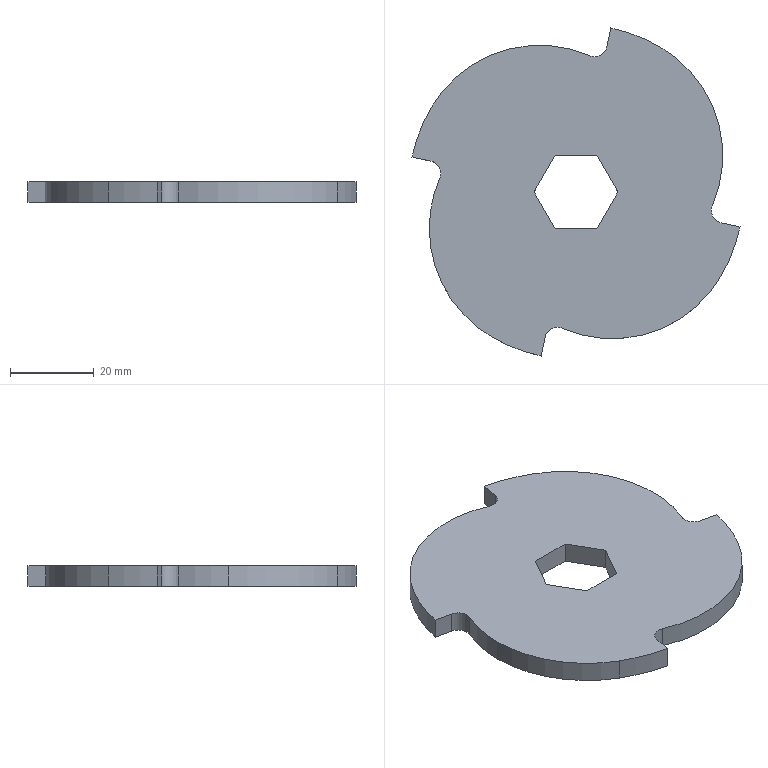Part | NX | 1 solid | 26 faces | box 78.252 x 78.252 x 5 mm | volume 21007 mm3 | cylinder 14 | plane 12 | commonest cylinder face diameters 6 x5 60 x5 80 x4
STEP:
#1=CARTESIAN_POINT('',(-35.,-8.66,5.));
#2=VERTEX_POINT('',#1);
#3=CARTESIAN_POINT('',(-20.,-34.641,5.));
#4=VERTEX_POINT('',#3);
#5=CARTESIAN_POINT('',(-5.,-8.66,5.));
#6=DIRECTION('',(0.,0.,1.));
#7=DIRECTION('',(1.,0.,0.));
#8=AXIS2_PLACEMENT_3D('',#5,#6,#7);
#9=CIRCLE('',#8,30.);
#10=EDGE_CURVE('',#2,#4,#9,.T.);
#11=ORIENTED_EDGE('',*,*,#10,.F.);
#12=CARTESIAN_POINT('',(-35.,-8.66,0.));
#13=VERTEX_POINT('',#12);
#14=CARTESIAN_POINT('',(-35.,-8.66,5.));
#15=DIRECTION('',(0.,0.,-1.));
#16=VECTOR('',#15,1.);
#17=LINE('',#14,#16);
#18=EDGE_CURVE('',#2,#13,#17,.T.);
#19=ORIENTED_EDGE('',*,*,#18,.T.);
#20=CARTESIAN_POINT('',(-20.,-34.641,0.));
#21=VERTEX_POINT('',#20);
#22=CARTESIAN_POINT('',(-5.,-8.66,0.));
#23=DIRECTION('',(0.,0.,1.));
#24=DIRECTION('',(1.,0.,0.));
#25=AXIS2_PLACEMENT_3D('',#22,#23,#24);
#26=CIRCLE('',#25,30.);
#27=EDGE_CURVE('',#13,#21,#26,.T.);
#28=ORIENTED_EDGE('',*,*,#27,.T.);
#29=CARTESIAN_POINT('',(-20.,-34.641,5.));
#30=DIRECTION('',(0.,0.,-1.));
#31=VECTOR('',#30,1.);
#32=LINE('',#29,#31);
#33=EDGE_CURVE('',#4,#21,#32,.T.);
#34=ORIENTED_EDGE('',*,*,#33,.F.);
#35=EDGE_LOOP('',(#11,#19,#28,#34));
#36=FACE_OUTER_BOUND('',#35,.T.);
#37=CARTESIAN_POINT('',(-5.,-8.66,5.));
#38=DIRECTION('',(0.,0.,-1.));
#39=DIRECTION('',(-1.,0.,0.));
#40=AXIS2_PLACEMENT_3D('',#37,#38,#39);
#41=CYLINDRICAL_SURFACE('',#40,30.);
#42=ADVANCED_FACE('',(#36),#41,.T.);
#43=CARTESIAN_POINT('',(32.291,-4.434,5.));
#44=VERTEX_POINT('',#43);
#45=CARTESIAN_POINT('',(32.537,-3.244,5.));
#46=VERTEX_POINT('',#45);
#47=CARTESIAN_POINT('',(35.291,-4.434,5.));
#48=DIRECTION('',(0.,0.,-1.));
#49=DIRECTION('',(1.,0.,0.));
#50=AXIS2_PLACEMENT_3D('',#47,#48,#49);
#51=CIRCLE('',#50,3.);
#52=EDGE_CURVE('',#44,#46,#51,.T.);
#53=ORIENTED_EDGE('',*,*,#52,.F.);
#54=CARTESIAN_POINT('',(32.291,-4.434,0.));
#55=VERTEX_POINT('',#54);
#56=CARTESIAN_POINT('',(32.291,-4.434,5.));
#57=DIRECTION('',(0.,0.,-1.));
#58=VECTOR('',#57,1.);
#59=LINE('',#56,#58);
#60=EDGE_CURVE('',#44,#55,#59,.T.);
#61=ORIENTED_EDGE('',*,*,#60,.T.);
#62=CARTESIAN_POINT('',(32.537,-3.244,0.));
#63=VERTEX_POINT('',#62);
#64=CARTESIAN_POINT('',(35.291,-4.434,0.));
#65=DIRECTION('',(0.,0.,-1.));
#66=DIRECTION('',(1.,0.,0.));
#67=AXIS2_PLACEMENT_3D('',#64,#65,#66);
#68=CIRCLE('',#67,3.);
#69=EDGE_CURVE('',#55,#63,#68,.T.);
#70=ORIENTED_EDGE('',*,*,#69,.T.);
#71=CARTESIAN_POINT('',(32.537,-3.244,5.));
#72=DIRECTION('',(0.,0.,-1.));
#73=VECTOR('',#72,1.);
#74=LINE('',#71,#73);
#75=EDGE_CURVE('',#46,#63,#74,.T.);
#76=ORIENTED_EDGE('',*,*,#75,.F.);
#77=EDGE_LOOP('',(#53,#61,#70,#76));
#78=FACE_OUTER_BOUND('',#77,.T.);
#79=CARTESIAN_POINT('',(35.291,-4.434,5.));
#80=DIRECTION('',(0.,0.,-1.));
#81=DIRECTION('',(-1.,0.,0.));
#82=AXIS2_PLACEMENT_3D('',#79,#80,#81);
#83=CYLINDRICAL_SURFACE('',#82,3.);
#84=ADVANCED_FACE('',(#78),#83,.F.);
#85=CARTESIAN_POINT('',(-3.244,-32.537,0.));
#86=VERTEX_POINT('',#85);
#87=CARTESIAN_POINT('',(34.641,-20.,0.));
#88=VERTEX_POINT('',#87);
#89=CARTESIAN_POINT('',(8.66,-5.,0.));
#90=DIRECTION('',(0.,0.,1.));
#91=DIRECTION('',(1.,0.,0.));
#92=AXIS2_PLACEMENT_3D('',#89,#90,#91);
#93=CIRCLE('',#92,30.);
#94=EDGE_CURVE('',#86,#88,#93,.T.);
#95=ORIENTED_EDGE('',*,*,#94,.T.);
#96=CARTESIAN_POINT('',(34.641,-20.,5.));
#97=VERTEX_POINT('',#96);
#98=CARTESIAN_POINT('',(34.641,-20.,5.));
#99=DIRECTION('',(0.,0.,-1.));
#100=VECTOR('',#99,1.);
#101=LINE('',#98,#100);
#102=EDGE_CURVE('',#97,#88,#101,.T.);
#103=ORIENTED_EDGE('',*,*,#102,.F.);
#104=CARTESIAN_POINT('',(-3.244,-32.537,5.));
#105=VERTEX_POINT('',#104);
#106=CARTESIAN_POINT('',(8.66,-5.,5.));
#107=DIRECTION('',(0.,0.,1.));
#108=DIRECTION('',(1.,0.,0.));
#109=AXIS2_PLACEMENT_3D('',#106,#107,#108);
#110=CIRCLE('',#109,30.);
#111=EDGE_CURVE('',#105,#97,#110,.T.);
#112=ORIENTED_EDGE('',*,*,#111,.F.);
#113=CARTESIAN_POINT('',(-3.244,-32.537,5.));
#114=DIRECTION('',(0.,0.,-1.));
#115=VECTOR('',#114,1.);
#116=LINE('',#113,#115);
#117=EDGE_CURVE('',#105,#86,#116,.T.);
#118=ORIENTED_EDGE('',*,*,#117,.T.);
#119=EDGE_LOOP('',(#95,#103,#112,#118));
#120=FACE_OUTER_BOUND('',#119,.T.);
#121=CARTESIAN_POINT('',(8.66,-5.,5.));
#122=DIRECTION('',(0.,0.,-1.));
#123=DIRECTION('',(-1.,0.,0.));
#124=AXIS2_PLACEMENT_3D('',#121,#122,#123);
#125=CYLINDRICAL_SURFACE('',#124,30.);
#126=ADVANCED_FACE('',(#120),#125,.T.);
#127=CARTESIAN_POINT('',(39.126,-8.316,0.));
#128=VERTEX_POINT('',#127);
#129=CARTESIAN_POINT('',(0.,0.,0.));
#130=DIRECTION('',(0.,0.,1.));
#131=DIRECTION('',(1.,0.,0.));
#132=AXIS2_PLACEMENT_3D('',#129,#130,#131);
#133=CIRCLE('',#132,40.);
#134=EDGE_CURVE('',#88,#128,#133,.T.);
#135=ORIENTED_EDGE('',*,*,#134,.T.);
#136=CARTESIAN_POINT('',(39.126,-8.316,5.));
#137=VERTEX_POINT('',#136);
#138=CARTESIAN_POINT('',(39.126,-8.316,5.));
#139=DIRECTION('',(0.,0.,-1.));
#140=VECTOR('',#139,1.);
#141=LINE('',#138,#140);
#142=EDGE_CURVE('',#137,#128,#141,.T.);
#143=ORIENTED_EDGE('',*,*,#142,.F.);
#144=CARTESIAN_POINT('',(0.,0.,5.));
#145=DIRECTION('',(0.,0.,1.));
#146=DIRECTION('',(1.,0.,0.));
#147=AXIS2_PLACEMENT_3D('',#144,#145,#146);
#148=CIRCLE('',#147,40.);
#149=EDGE_CURVE('',#97,#137,#148,.T.);
#150=ORIENTED_EDGE('',*,*,#149,.F.);
#151=ORIENTED_EDGE('',*,*,#102,.T.);
#152=EDGE_LOOP('',(#135,#143,#150,#151));
#153=FACE_OUTER_BOUND('',#152,.T.);
#154=CARTESIAN_POINT('',(0.,0.,5.));
#155=DIRECTION('',(0.,0.,-1.));
#156=DIRECTION('',(-1.,0.,0.));
#157=AXIS2_PLACEMENT_3D('',#154,#155,#156);
#158=CYLINDRICAL_SURFACE('',#157,40.);
#159=ADVANCED_FACE('',(#153),#158,.T.);
#160=CARTESIAN_POINT('',(34.667,-7.369,0.));
#161=VERTEX_POINT('',#160);
#162=CARTESIAN_POINT('',(17.574,-3.736,0.));
#163=DIRECTION('',(0.9781,-0.2079,0.));
#164=VECTOR('',#163,1.);
#165=LINE('',#162,#164);
#166=EDGE_CURVE('',#161,#128,#165,.T.);
#167=ORIENTED_EDGE('',*,*,#166,.F.);
#168=CARTESIAN_POINT('',(34.667,-7.369,5.));
#169=VERTEX_POINT('',#168);
#170=CARTESIAN_POINT('',(34.667,-7.369,5.));
#171=DIRECTION('',(0.,0.,-1.));
#172=VECTOR('',#171,1.);
#173=LINE('',#170,#172);
#174=EDGE_CURVE('',#169,#161,#173,.T.);
#175=ORIENTED_EDGE('',*,*,#174,.F.);
#176=CARTESIAN_POINT('',(17.574,-3.736,5.));
#177=DIRECTION('',(0.9781,-0.2079,0.));
#178=VECTOR('',#177,1.);
#179=LINE('',#176,#178);
#180=EDGE_CURVE('',#169,#137,#179,.T.);
#181=ORIENTED_EDGE('',*,*,#180,.T.);
#182=ORIENTED_EDGE('',*,*,#142,.T.);
#183=EDGE_LOOP('',(#167,#175,#181,#182));
#184=FACE_OUTER_BOUND('',#183,.T.);
#185=CARTESIAN_POINT('',(17.574,-3.736,5.));
#186=DIRECTION('',(0.2079,0.9781,0.));
#187=DIRECTION('',(-0.9781,0.2079,0.));
#188=AXIS2_PLACEMENT_3D('',#185,#186,#187);
#189=PLANE('',#188);
#190=ADVANCED_FACE('',(#184),#189,.T.);
#191=ORIENTED_EDGE('',*,*,#60,.F.);
#192=CARTESIAN_POINT('',(35.291,-4.434,5.));
#193=DIRECTION('',(0.,0.,-1.));
#194=DIRECTION('',(1.,0.,0.));
#195=AXIS2_PLACEMENT_3D('',#192,#193,#194);
#196=CIRCLE('',#195,3.);
#197=EDGE_CURVE('',#169,#44,#196,.T.);
#198=ORIENTED_EDGE('',*,*,#197,.F.);
#199=ORIENTED_EDGE('',*,*,#174,.T.);
#200=CARTESIAN_POINT('',(35.291,-4.434,0.));
#201=DIRECTION('',(0.,0.,-1.));
#202=DIRECTION('',(1.,0.,0.));
#203=AXIS2_PLACEMENT_3D('',#200,#201,#202);
#204=CIRCLE('',#203,3.);
#205=EDGE_CURVE('',#161,#55,#204,.T.);
#206=ORIENTED_EDGE('',*,*,#205,.T.);
#207=EDGE_LOOP('',(#191,#198,#199,#206));
#208=FACE_OUTER_BOUND('',#207,.T.);
#209=CARTESIAN_POINT('',(35.291,-4.434,5.));
#210=DIRECTION('',(0.,0.,-1.));
#211=DIRECTION('',(-1.,0.,0.));
#212=AXIS2_PLACEMENT_3D('',#209,#210,#211);
#213=CYLINDRICAL_SURFACE('',#212,3.);
#214=ADVANCED_FACE('',(#208),#213,.F.);
#215=CARTESIAN_POINT('',(20.,34.641,0.));
#216=VERTEX_POINT('',#215);
#217=CARTESIAN_POINT('',(5.,8.66,0.));
#218=DIRECTION('',(0.,0.,1.));
#219=DIRECTION('',(1.,0.,0.));
#220=AXIS2_PLACEMENT_3D('',#217,#218,#219);
#221=CIRCLE('',#220,30.);
#222=EDGE_CURVE('',#63,#216,#221,.T.);
#223=ORIENTED_EDGE('',*,*,#222,.T.);
#224=CARTESIAN_POINT('',(20.,34.641,5.));
#225=VERTEX_POINT('',#224);
#226=CARTESIAN_POINT('',(20.,34.641,5.));
#227=DIRECTION('',(0.,0.,-1.));
#228=VECTOR('',#227,1.);
#229=LINE('',#226,#228);
#230=EDGE_CURVE('',#225,#216,#229,.T.);
#231=ORIENTED_EDGE('',*,*,#230,.F.);
#232=CARTESIAN_POINT('',(5.,8.66,5.));
#233=DIRECTION('',(0.,0.,1.));
#234=DIRECTION('',(1.,0.,0.));
#235=AXIS2_PLACEMENT_3D('',#232,#233,#234);
#236=CIRCLE('',#235,30.);
#237=EDGE_CURVE('',#46,#225,#236,.T.);
#238=ORIENTED_EDGE('',*,*,#237,.F.);
#239=ORIENTED_EDGE('',*,*,#75,.T.);
#240=EDGE_LOOP('',(#223,#231,#238,#239));
#241=FACE_OUTER_BOUND('',#240,.T.);
#242=CARTESIAN_POINT('',(5.,8.66,5.));
#243=DIRECTION('',(0.,0.,-1.));
#244=DIRECTION('',(-1.,0.,0.));
#245=AXIS2_PLACEMENT_3D('',#242,#243,#244);
#246=CYLINDRICAL_SURFACE('',#245,30.);
#247=ADVANCED_FACE('',(#241),#246,.T.);
#248=CARTESIAN_POINT('',(8.316,39.126,0.));
#249=VERTEX_POINT('',#248);
#250=CARTESIAN_POINT('',(0.,0.,0.));
#251=DIRECTION('',(0.,0.,1.));
#252=DIRECTION('',(1.,0.,0.));
#253=AXIS2_PLACEMENT_3D('',#250,#251,#252);
#254=CIRCLE('',#253,40.);
#255=EDGE_CURVE('',#216,#249,#254,.T.);
#256=ORIENTED_EDGE('',*,*,#255,.T.);
#257=CARTESIAN_POINT('',(8.316,39.126,5.));
#258=VERTEX_POINT('',#257);
#259=CARTESIAN_POINT('',(8.316,39.126,5.));
#260=DIRECTION('',(0.,0.,-1.));
#261=VECTOR('',#260,1.);
#262=LINE('',#259,#261);
#263=EDGE_CURVE('',#258,#249,#262,.T.);
#264=ORIENTED_EDGE('',*,*,#263,.F.);
#265=CARTESIAN_POINT('',(0.,0.,5.));
#266=DIRECTION('',(0.,0.,1.));
#267=DIRECTION('',(1.,0.,0.));
#268=AXIS2_PLACEMENT_3D('',#265,#266,#267);
#269=CIRCLE('',#268,40.);
#270=EDGE_CURVE('',#225,#258,#269,.T.);
#271=ORIENTED_EDGE('',*,*,#270,.F.);
#272=ORIENTED_EDGE('',*,*,#230,.T.);
#273=EDGE_LOOP('',(#256,#264,#271,#272));
#274=FACE_OUTER_BOUND('',#273,.T.);
#275=CARTESIAN_POINT('',(0.,0.,5.));
#276=DIRECTION('',(0.,0.,-1.));
#277=DIRECTION('',(-1.,0.,0.));
#278=AXIS2_PLACEMENT_3D('',#275,#276,#277);
#279=CYLINDRICAL_SURFACE('',#278,40.);
#280=ADVANCED_FACE('',(#274),#279,.T.);
#281=CARTESIAN_POINT('',(7.369,34.667,0.));
#282=VERTEX_POINT('',#281);
#283=CARTESIAN_POINT('',(-17.016,-80.056,0.));
#284=DIRECTION('',(0.2079,0.9781,0.));
#285=VECTOR('',#284,1.);
#286=LINE('',#283,#285);
#287=EDGE_CURVE('',#282,#249,#286,.T.);
#288=ORIENTED_EDGE('',*,*,#287,.F.);
#289=CARTESIAN_POINT('',(7.369,34.667,5.));
#290=VERTEX_POINT('',#289);
#291=CARTESIAN_POINT('',(7.369,34.667,5.));
#292=DIRECTION('',(0.,0.,-1.));
#293=VECTOR('',#292,1.);
#294=LINE('',#291,#293);
#295=EDGE_CURVE('',#290,#282,#294,.T.);
#296=ORIENTED_EDGE('',*,*,#295,.F.);
#297=CARTESIAN_POINT('',(-17.016,-80.056,5.));
#298=DIRECTION('',(0.2079,0.9781,0.));
#299=VECTOR('',#298,1.);
#300=LINE('',#297,#299);
#301=EDGE_CURVE('',#290,#258,#300,.T.);
#302=ORIENTED_EDGE('',*,*,#301,.T.);
#303=ORIENTED_EDGE('',*,*,#263,.T.);
#304=EDGE_LOOP('',(#288,#296,#302,#303));
#305=FACE_OUTER_BOUND('',#304,.T.);
#306=CARTESIAN_POINT('',(-17.016,-80.056,5.));
#307=DIRECTION('',(-0.9781,0.2079,0.));
#308=DIRECTION('',(-0.2079,-0.9781,0.));
#309=AXIS2_PLACEMENT_3D('',#306,#307,#308);
#310=PLANE('',#309);
#311=ADVANCED_FACE('',(#305),#310,.T.);
#312=CARTESIAN_POINT('',(3.244,32.537,0.));
#313=VERTEX_POINT('',#312);
#314=CARTESIAN_POINT('',(4.434,35.291,0.));
#315=DIRECTION('',(0.,0.,-1.));
#316=DIRECTION('',(1.,0.,0.));
#317=AXIS2_PLACEMENT_3D('',#314,#315,#316);
#318=CIRCLE('',#317,3.);
#319=EDGE_CURVE('',#282,#313,#318,.T.);
#320=ORIENTED_EDGE('',*,*,#319,.T.);
#321=CARTESIAN_POINT('',(3.244,32.537,5.));
#322=VERTEX_POINT('',#321);
#323=CARTESIAN_POINT('',(3.244,32.537,5.));
#324=DIRECTION('',(0.,0.,-1.));
#325=VECTOR('',#324,1.);
#326=LINE('',#323,#325);
#327=EDGE_CURVE('',#322,#313,#326,.T.);
#328=ORIENTED_EDGE('',*,*,#327,.F.);
#329=CARTESIAN_POINT('',(4.434,35.291,5.));
#330=DIRECTION('',(0.,0.,-1.));
#331=DIRECTION('',(1.,0.,0.));
#332=AXIS2_PLACEMENT_3D('',#329,#330,#331);
#333=CIRCLE('',#332,3.);
#334=EDGE_CURVE('',#290,#322,#333,.T.);
#335=ORIENTED_EDGE('',*,*,#334,.F.);
#336=ORIENTED_EDGE('',*,*,#295,.T.);
#337=EDGE_LOOP('',(#320,#328,#335,#336));
#338=FACE_OUTER_BOUND('',#337,.T.);
#339=CARTESIAN_POINT('',(4.434,35.291,5.));
#340=DIRECTION('',(0.,0.,-1.));
#341=DIRECTION('',(-1.,0.,0.));
#342=AXIS2_PLACEMENT_3D('',#339,#340,#341);
#343=CYLINDRICAL_SURFACE('',#342,3.);
#344=ADVANCED_FACE('',(#338),#343,.F.);
#345=CARTESIAN_POINT('',(-34.641,20.,0.));
#346=VERTEX_POINT('',#345);
#347=CARTESIAN_POINT('',(-8.66,5.,0.));
#348=DIRECTION('',(0.,0.,1.));
#349=DIRECTION('',(1.,0.,0.));
#350=AXIS2_PLACEMENT_3D('',#347,#348,#349);
#351=CIRCLE('',#350,30.);
#352=EDGE_CURVE('',#313,#346,#351,.T.);
#353=ORIENTED_EDGE('',*,*,#352,.T.);
#354=CARTESIAN_POINT('',(-34.641,20.,5.));
#355=VERTEX_POINT('',#354);
#356=CARTESIAN_POINT('',(-34.641,20.,5.));
#357=DIRECTION('',(0.,0.,-1.));
#358=VECTOR('',#357,1.);
#359=LINE('',#356,#358);
#360=EDGE_CURVE('',#355,#346,#359,.T.);
#361=ORIENTED_EDGE('',*,*,#360,.F.);
#362=CARTESIAN_POINT('',(-8.66,5.,5.));
#363=DIRECTION('',(0.,0.,1.));
#364=DIRECTION('',(1.,0.,0.));
#365=AXIS2_PLACEMENT_3D('',#362,#363,#364);
#366=CIRCLE('',#365,30.);
#367=EDGE_CURVE('',#322,#355,#366,.T.);
#368=ORIENTED_EDGE('',*,*,#367,.F.);
#369=ORIENTED_EDGE('',*,*,#327,.T.);
#370=EDGE_LOOP('',(#353,#361,#368,#369));
#371=FACE_OUTER_BOUND('',#370,.T.);
#372=CARTESIAN_POINT('',(-8.66,5.,5.));
#373=DIRECTION('',(0.,0.,-1.));
#374=DIRECTION('',(-1.,0.,0.));
#375=AXIS2_PLACEMENT_3D('',#372,#373,#374);
#376=CYLINDRICAL_SURFACE('',#375,30.);
#377=ADVANCED_FACE('',(#371),#376,.T.);
#378=CARTESIAN_POINT('',(-39.126,8.316,0.));
#379=VERTEX_POINT('',#378);
#380=CARTESIAN_POINT('',(0.,0.,0.));
#381=DIRECTION('',(0.,0.,1.));
#382=DIRECTION('',(1.,0.,0.));
#383=AXIS2_PLACEMENT_3D('',#380,#381,#382);
#384=CIRCLE('',#383,40.);
#385=EDGE_CURVE('',#346,#379,#384,.T.);
#386=ORIENTED_EDGE('',*,*,#385,.T.);
#387=CARTESIAN_POINT('',(-39.126,8.316,5.));
#388=VERTEX_POINT('',#387);
#389=CARTESIAN_POINT('',(-39.126,8.316,5.));
#390=DIRECTION('',(0.,0.,-1.));
#391=VECTOR('',#390,1.);
#392=LINE('',#389,#391);
#393=EDGE_CURVE('',#388,#379,#392,.T.);
#394=ORIENTED_EDGE('',*,*,#393,.F.);
#395=CARTESIAN_POINT('',(0.,0.,5.));
#396=DIRECTION('',(0.,0.,1.));
#397=DIRECTION('',(1.,0.,0.));
#398=AXIS2_PLACEMENT_3D('',#395,#396,#397);
#399=CIRCLE('',#398,40.);
#400=EDGE_CURVE('',#355,#388,#399,.T.);
#401=ORIENTED_EDGE('',*,*,#400,.F.);
#402=ORIENTED_EDGE('',*,*,#360,.T.);
#403=EDGE_LOOP('',(#386,#394,#401,#402));
#404=FACE_OUTER_BOUND('',#403,.T.);
#405=CARTESIAN_POINT('',(0.,0.,5.));
#406=DIRECTION('',(0.,0.,-1.));
#407=DIRECTION('',(-1.,0.,0.));
#408=AXIS2_PLACEMENT_3D('',#405,#406,#407);
#409=CYLINDRICAL_SURFACE('',#408,40.);
#410=ADVANCED_FACE('',(#404),#409,.T.);
#411=CARTESIAN_POINT('',(-34.667,7.369,0.));
#412=VERTEX_POINT('',#411);
#413=CARTESIAN_POINT('',(17.574,-3.736,0.));
#414=DIRECTION('',(-0.9781,0.2079,0.));
#415=VECTOR('',#414,1.);
#416=LINE('',#413,#415);
#417=EDGE_CURVE('',#412,#379,#416,.T.);
#418=ORIENTED_EDGE('',*,*,#417,.F.);
#419=CARTESIAN_POINT('',(-34.667,7.369,5.));
#420=VERTEX_POINT('',#419);
#421=CARTESIAN_POINT('',(-34.667,7.369,5.));
#422=DIRECTION('',(0.,0.,-1.));
#423=VECTOR('',#422,1.);
#424=LINE('',#421,#423);
#425=EDGE_CURVE('',#420,#412,#424,.T.);
#426=ORIENTED_EDGE('',*,*,#425,.F.);
#427=CARTESIAN_POINT('',(17.574,-3.736,5.));
#428=DIRECTION('',(-0.9781,0.2079,0.));
#429=VECTOR('',#428,1.);
#430=LINE('',#427,#429);
#431=EDGE_CURVE('',#420,#388,#430,.T.);
#432=ORIENTED_EDGE('',*,*,#431,.T.);
#433=ORIENTED_EDGE('',*,*,#393,.T.);
#434=EDGE_LOOP('',(#418,#426,#432,#433));
#435=FACE_OUTER_BOUND('',#434,.T.);
#436=CARTESIAN_POINT('',(17.574,-3.736,5.));
#437=DIRECTION('',(-0.2079,-0.9781,0.));
#438=DIRECTION('',(0.9781,-0.2079,0.));
#439=AXIS2_PLACEMENT_3D('',#436,#437,#438);
#440=PLANE('',#439);
#441=ADVANCED_FACE('',(#435),#440,.T.);
#442=CARTESIAN_POINT('',(-32.537,3.244,0.));
#443=VERTEX_POINT('',#442);
#444=CARTESIAN_POINT('',(-35.291,4.434,0.));
#445=DIRECTION('',(0.,0.,-1.));
#446=DIRECTION('',(1.,0.,0.));
#447=AXIS2_PLACEMENT_3D('',#444,#445,#446);
#448=CIRCLE('',#447,3.);
#449=EDGE_CURVE('',#412,#443,#448,.T.);
#450=ORIENTED_EDGE('',*,*,#449,.T.);
#451=CARTESIAN_POINT('',(-32.537,3.244,5.));
#452=VERTEX_POINT('',#451);
#453=CARTESIAN_POINT('',(-32.537,3.244,5.));
#454=DIRECTION('',(0.,0.,-1.));
#455=VECTOR('',#454,1.);
#456=LINE('',#453,#455);
#457=EDGE_CURVE('',#452,#443,#456,.T.);
#458=ORIENTED_EDGE('',*,*,#457,.F.);
#459=CARTESIAN_POINT('',(-35.291,4.434,5.));
#460=DIRECTION('',(0.,0.,-1.));
#461=DIRECTION('',(1.,0.,0.));
#462=AXIS2_PLACEMENT_3D('',#459,#460,#461);
#463=CIRCLE('',#462,3.);
#464=EDGE_CURVE('',#420,#452,#463,.T.);
#465=ORIENTED_EDGE('',*,*,#464,.F.);
#466=ORIENTED_EDGE('',*,*,#425,.T.);
#467=EDGE_LOOP('',(#450,#458,#465,#466));
#468=FACE_OUTER_BOUND('',#467,.T.);
#469=CARTESIAN_POINT('',(-35.291,4.434,5.));
#470=DIRECTION('',(0.,0.,-1.));
#471=DIRECTION('',(-1.,0.,0.));
#472=AXIS2_PLACEMENT_3D('',#469,#470,#471);
#473=CYLINDRICAL_SURFACE('',#472,3.);
#474=ADVANCED_FACE('',(#468),#473,.F.);
#475=ORIENTED_EDGE('',*,*,#18,.F.);
#476=CARTESIAN_POINT('',(-5.,-8.66,5.));
#477=DIRECTION('',(0.,0.,1.));
#478=DIRECTION('',(1.,0.,0.));
#479=AXIS2_PLACEMENT_3D('',#476,#477,#478);
#480=CIRCLE('',#479,30.);
#481=EDGE_CURVE('',#452,#2,#480,.T.);
#482=ORIENTED_EDGE('',*,*,#481,.F.);
#483=ORIENTED_EDGE('',*,*,#457,.T.);
#484=CARTESIAN_POINT('',(-5.,-8.66,0.));
#485=DIRECTION('',(0.,0.,1.));
#486=DIRECTION('',(1.,0.,0.));
#487=AXIS2_PLACEMENT_3D('',#484,#485,#486);
#488=CIRCLE('',#487,30.);
#489=EDGE_CURVE('',#443,#13,#488,.T.);
#490=ORIENTED_EDGE('',*,*,#489,.T.);
#491=EDGE_LOOP('',(#475,#482,#483,#490));
#492=FACE_OUTER_BOUND('',#491,.T.);
#493=CARTESIAN_POINT('',(-5.,-8.66,5.));
#494=DIRECTION('',(0.,0.,-1.));
#495=DIRECTION('',(-1.,0.,0.));
#496=AXIS2_PLACEMENT_3D('',#493,#494,#495);
#497=CYLINDRICAL_SURFACE('',#496,30.);
#498=ADVANCED_FACE('',(#492),#497,.T.);
#499=CARTESIAN_POINT('',(-8.316,-39.126,0.));
#500=VERTEX_POINT('',#499);
#501=CARTESIAN_POINT('',(0.,0.,0.));
#502=DIRECTION('',(0.,0.,1.));
#503=DIRECTION('',(1.,0.,0.));
#504=AXIS2_PLACEMENT_3D('',#501,#502,#503);
#505=CIRCLE('',#504,40.);
#506=EDGE_CURVE('',#21,#500,#505,.T.);
#507=ORIENTED_EDGE('',*,*,#506,.T.);
#508=CARTESIAN_POINT('',(-8.316,-39.126,5.));
#509=VERTEX_POINT('',#508);
#510=CARTESIAN_POINT('',(-8.316,-39.126,5.));
#511=DIRECTION('',(0.,0.,-1.));
#512=VECTOR('',#511,1.);
#513=LINE('',#510,#512);
#514=EDGE_CURVE('',#509,#500,#513,.T.);
#515=ORIENTED_EDGE('',*,*,#514,.F.);
#516=CARTESIAN_POINT('',(0.,0.,5.));
#517=DIRECTION('',(0.,0.,1.));
#518=DIRECTION('',(1.,0.,0.));
#519=AXIS2_PLACEMENT_3D('',#516,#517,#518);
#520=CIRCLE('',#519,40.);
#521=EDGE_CURVE('',#4,#509,#520,.T.);
#522=ORIENTED_EDGE('',*,*,#521,.F.);
#523=ORIENTED_EDGE('',*,*,#33,.T.);
#524=EDGE_LOOP('',(#507,#515,#522,#523));
#525=FACE_OUTER_BOUND('',#524,.T.);
#526=CARTESIAN_POINT('',(0.,0.,5.));
#527=DIRECTION('',(0.,0.,-1.));
#528=DIRECTION('',(-1.,0.,0.));
#529=AXIS2_PLACEMENT_3D('',#526,#527,#528);
#530=CYLINDRICAL_SURFACE('',#529,40.);
#531=ADVANCED_FACE('',(#525),#530,.T.);
#532=CARTESIAN_POINT('',(-7.369,-34.667,0.));
#533=VERTEX_POINT('',#532);
#534=CARTESIAN_POINT('',(-17.016,-80.056,0.));
#535=DIRECTION('',(-0.2079,-0.9781,0.));
#536=VECTOR('',#535,1.);
#537=LINE('',#534,#536);
#538=EDGE_CURVE('',#533,#500,#537,.T.);
#539=ORIENTED_EDGE('',*,*,#538,.F.);
#540=CARTESIAN_POINT('',(-7.369,-34.667,5.));
#541=VERTEX_POINT('',#540);
#542=CARTESIAN_POINT('',(-7.369,-34.667,5.));
#543=DIRECTION('',(0.,0.,-1.));
#544=VECTOR('',#543,1.);
#545=LINE('',#542,#544);
#546=EDGE_CURVE('',#541,#533,#545,.T.);
#547=ORIENTED_EDGE('',*,*,#546,.F.);
#548=CARTESIAN_POINT('',(-17.016,-80.056,5.));
#549=DIRECTION('',(-0.2079,-0.9781,0.));
#550=VECTOR('',#549,1.);
#551=LINE('',#548,#550);
#552=EDGE_CURVE('',#541,#509,#551,.T.);
#553=ORIENTED_EDGE('',*,*,#552,.T.);
#554=ORIENTED_EDGE('',*,*,#514,.T.);
#555=EDGE_LOOP('',(#539,#547,#553,#554));
#556=FACE_OUTER_BOUND('',#555,.T.);
#557=CARTESIAN_POINT('',(-17.016,-80.056,5.));
#558=DIRECTION('',(0.9781,-0.2079,0.));
#559=DIRECTION('',(0.2079,0.9781,0.));
#560=AXIS2_PLACEMENT_3D('',#557,#558,#559);
#561=PLANE('',#560);
#562=ADVANCED_FACE('',(#556),#561,.T.);
#563=CARTESIAN_POINT('',(5.,-8.66,0.));
#564=VERTEX_POINT('',#563);
#565=CARTESIAN_POINT('',(10.,0.,0.));
#566=VERTEX_POINT('',#565);
#567=CARTESIAN_POINT('',(-28.643,-66.932,0.));
#568=DIRECTION('',(0.5,0.866,0.));
#569=VECTOR('',#568,1.);
#570=LINE('',#567,#569);
#571=EDGE_CURVE('',#564,#566,#570,.T.);
#572=ORIENTED_EDGE('',*,*,#571,.F.);
#573=CARTESIAN_POINT('',(5.,-8.66,5.));
#574=VERTEX_POINT('',#573);
#575=CARTESIAN_POINT('',(5.,-8.66,5.));
#576=DIRECTION('',(0.,0.,-1.));
#577=VECTOR('',#576,1.);
#578=LINE('',#575,#577);
#579=EDGE_CURVE('',#574,#564,#578,.T.);
#580=ORIENTED_EDGE('',*,*,#579,.F.);
#581=CARTESIAN_POINT('',(10.,0.,5.));
#582=VERTEX_POINT('',#581);
#583=CARTESIAN_POINT('',(-28.643,-66.932,5.));
#584=DIRECTION('',(0.5,0.866,0.));
#585=VECTOR('',#584,1.);
#586=LINE('',#583,#585);
#587=EDGE_CURVE('',#574,#582,#586,.T.);
#588=ORIENTED_EDGE('',*,*,#587,.T.);
#589=CARTESIAN_POINT('',(10.,0.,5.));
#590=DIRECTION('',(0.,0.,-1.));
#591=VECTOR('',#590,1.);
#592=LINE('',#589,#591);
#593=EDGE_CURVE('',#582,#566,#592,.T.);
#594=ORIENTED_EDGE('',*,*,#593,.T.);
#595=EDGE_LOOP('',(#572,#580,#588,#594));
#596=FACE_OUTER_BOUND('',#595,.T.);
#597=CARTESIAN_POINT('',(-28.643,-66.932,5.));
#598=DIRECTION('',(-0.866,0.5,0.));
#599=DIRECTION('',(-0.5,-0.866,0.));
#600=AXIS2_PLACEMENT_3D('',#597,#598,#599);
#601=PLANE('',#600);
#602=ADVANCED_FACE('',(#596),#601,.T.);
#603=CARTESIAN_POINT('',(-5.,-8.66,0.));
#604=VERTEX_POINT('',#603);
#605=CARTESIAN_POINT('',(0.5581,-8.66,0.));
#606=DIRECTION('',(1.,0.,0.));
#607=VECTOR('',#606,1.);
#608=LINE('',#605,#607);
#609=EDGE_CURVE('',#604,#564,#608,.T.);
#610=ORIENTED_EDGE('',*,*,#609,.F.);
#611=CARTESIAN_POINT('',(-5.,-8.66,5.));
#612=VERTEX_POINT('',#611);
#613=CARTESIAN_POINT('',(-5.,-8.66,5.));
#614=DIRECTION('',(0.,0.,-1.));
#615=VECTOR('',#614,1.);
#616=LINE('',#613,#615);
#617=EDGE_CURVE('',#612,#604,#616,.T.);
#618=ORIENTED_EDGE('',*,*,#617,.F.);
#619=CARTESIAN_POINT('',(0.5581,-8.66,5.));
#620=DIRECTION('',(1.,0.,0.));
#621=VECTOR('',#620,1.);
#622=LINE('',#619,#621);
#623=EDGE_CURVE('',#612,#574,#622,.T.);
#624=ORIENTED_EDGE('',*,*,#623,.T.);
#625=ORIENTED_EDGE('',*,*,#579,.T.);
#626=EDGE_LOOP('',(#610,#618,#624,#625));
#627=FACE_OUTER_BOUND('',#626,.T.);
#628=CARTESIAN_POINT('',(0.5581,-8.66,5.));
#629=DIRECTION('',(0.,1.,0.));
#630=DIRECTION('',(-1.,0.,0.));
#631=AXIS2_PLACEMENT_3D('',#628,#629,#630);
#632=PLANE('',#631);
#633=ADVANCED_FACE('',(#627),#632,.T.);
#634=CARTESIAN_POINT('',(-10.,0.,0.));
#635=VERTEX_POINT('',#634);
#636=CARTESIAN_POINT('',(28.922,-67.415,0.));
#637=DIRECTION('',(0.5,-0.866,0.));
#638=VECTOR('',#637,1.);
#639=LINE('',#636,#638);
#640=EDGE_CURVE('',#635,#604,#639,.T.);
#641=ORIENTED_EDGE('',*,*,#640,.F.);
#642=CARTESIAN_POINT('',(-10.,0.,5.));
#643=VERTEX_POINT('',#642);
#644=CARTESIAN_POINT('',(-10.,0.,5.));
#645=DIRECTION('',(0.,0.,-1.));
#646=VECTOR('',#645,1.);
#647=LINE('',#644,#646);
#648=EDGE_CURVE('',#643,#635,#647,.T.);
#649=ORIENTED_EDGE('',*,*,#648,.F.);
#650=CARTESIAN_POINT('',(28.922,-67.415,5.));
#651=DIRECTION('',(0.5,-0.866,0.));
#652=VECTOR('',#651,1.);
#653=LINE('',#650,#652);
#654=EDGE_CURVE('',#643,#612,#653,.T.);
#655=ORIENTED_EDGE('',*,*,#654,.T.);
#656=ORIENTED_EDGE('',*,*,#617,.T.);
#657=EDGE_LOOP('',(#641,#649,#655,#656));
#658=FACE_OUTER_BOUND('',#657,.T.);
#659=CARTESIAN_POINT('',(28.922,-67.415,5.));
#660=DIRECTION('',(0.866,0.5,0.));
#661=DIRECTION('',(-0.5,0.866,0.));
#662=AXIS2_PLACEMENT_3D('',#659,#660,#661);
#663=PLANE('',#662);
#664=ADVANCED_FACE('',(#658),#663,.T.);
#665=CARTESIAN_POINT('',(-5.,8.66,0.));
#666=VERTEX_POINT('',#665);
#667=CARTESIAN_POINT('',(-43.643,-58.272,0.));
#668=DIRECTION('',(-0.5,-0.866,0.));
#669=VECTOR('',#668,1.);
#670=LINE('',#667,#669);
#671=EDGE_CURVE('',#666,#635,#670,.T.);
#672=ORIENTED_EDGE('',*,*,#671,.F.);
#673=CARTESIAN_POINT('',(-5.,8.66,5.));
#674=VERTEX_POINT('',#673);
#675=CARTESIAN_POINT('',(-5.,8.66,5.));
#676=DIRECTION('',(0.,0.,-1.));
#677=VECTOR('',#676,1.);
#678=LINE('',#675,#677);
#679=EDGE_CURVE('',#674,#666,#678,.T.);
#680=ORIENTED_EDGE('',*,*,#679,.F.);
#681=CARTESIAN_POINT('',(-43.643,-58.272,5.));
#682=DIRECTION('',(-0.5,-0.866,0.));
#683=VECTOR('',#682,1.);
#684=LINE('',#681,#683);
#685=EDGE_CURVE('',#674,#643,#684,.T.);
#686=ORIENTED_EDGE('',*,*,#685,.T.);
#687=ORIENTED_EDGE('',*,*,#648,.T.);
#688=EDGE_LOOP('',(#672,#680,#686,#687));
#689=FACE_OUTER_BOUND('',#688,.T.);
#690=CARTESIAN_POINT('',(-43.643,-58.272,5.));
#691=DIRECTION('',(0.866,-0.5,0.));
#692=DIRECTION('',(0.5,0.866,0.));
#693=AXIS2_PLACEMENT_3D('',#690,#691,#692);
#694=PLANE('',#693);
#695=ADVANCED_FACE('',(#689),#694,.T.);
#696=CARTESIAN_POINT('',(5.,8.66,0.));
#697=VERTEX_POINT('',#696);
#698=CARTESIAN_POINT('',(0.5581,8.66,0.));
#699=DIRECTION('',(-1.,0.,0.));
#700=VECTOR('',#699,1.);
#701=LINE('',#698,#700);
#702=EDGE_CURVE('',#697,#666,#701,.T.);
#703=ORIENTED_EDGE('',*,*,#702,.F.);
#704=CARTESIAN_POINT('',(5.,8.66,5.));
#705=VERTEX_POINT('',#704);
#706=CARTESIAN_POINT('',(5.,8.66,5.));
#707=DIRECTION('',(0.,0.,-1.));
#708=VECTOR('',#707,1.);
#709=LINE('',#706,#708);
#710=EDGE_CURVE('',#705,#697,#709,.T.);
#711=ORIENTED_EDGE('',*,*,#710,.F.);
#712=CARTESIAN_POINT('',(0.5581,8.66,5.));
#713=DIRECTION('',(-1.,0.,0.));
#714=VECTOR('',#713,1.);
#715=LINE('',#712,#714);
#716=EDGE_CURVE('',#705,#674,#715,.T.);
#717=ORIENTED_EDGE('',*,*,#716,.T.);
#718=ORIENTED_EDGE('',*,*,#679,.T.);
#719=EDGE_LOOP('',(#703,#711,#717,#718));
#720=FACE_OUTER_BOUND('',#719,.T.);
#721=CARTESIAN_POINT('',(0.5581,8.66,5.));
#722=DIRECTION('',(0.,-1.,0.));
#723=DIRECTION('',(1.,0.,0.));
#724=AXIS2_PLACEMENT_3D('',#721,#722,#723);
#725=PLANE('',#724);
#726=ADVANCED_FACE('',(#720),#725,.T.);
#727=CARTESIAN_POINT('',(43.922,-58.755,0.));
#728=DIRECTION('',(-0.5,0.866,0.));
#729=VECTOR('',#728,1.);
#730=LINE('',#727,#729);
#731=EDGE_CURVE('',#566,#697,#730,.T.);
#732=ORIENTED_EDGE('',*,*,#731,.F.);
#733=ORIENTED_EDGE('',*,*,#593,.F.);
#734=CARTESIAN_POINT('',(43.922,-58.755,5.));
#735=DIRECTION('',(-0.5,0.866,0.));
#736=VECTOR('',#735,1.);
#737=LINE('',#734,#736);
#738=EDGE_CURVE('',#582,#705,#737,.T.);
#739=ORIENTED_EDGE('',*,*,#738,.T.);
#740=ORIENTED_EDGE('',*,*,#710,.T.);
#741=EDGE_LOOP('',(#732,#733,#739,#740));
#742=FACE_OUTER_BOUND('',#741,.T.);
#743=CARTESIAN_POINT('',(43.922,-58.755,5.));
#744=DIRECTION('',(-0.866,-0.5,0.));
#745=DIRECTION('',(0.5,-0.866,0.));
#746=AXIS2_PLACEMENT_3D('',#743,#744,#745);
#747=PLANE('',#746);
#748=ADVANCED_FACE('',(#742),#747,.T.);
#749=CARTESIAN_POINT('',(-4.434,-35.291,0.));
#750=DIRECTION('',(0.,0.,-1.));
#751=DIRECTION('',(1.,0.,0.));
#752=AXIS2_PLACEMENT_3D('',#749,#750,#751);
#753=CIRCLE('',#752,3.);
#754=EDGE_CURVE('',#533,#86,#753,.T.);
#755=ORIENTED_EDGE('',*,*,#754,.T.);
#756=ORIENTED_EDGE('',*,*,#117,.F.);
#757=CARTESIAN_POINT('',(-4.434,-35.291,5.));
#758=DIRECTION('',(0.,0.,-1.));
#759=DIRECTION('',(1.,0.,0.));
#760=AXIS2_PLACEMENT_3D('',#757,#758,#759);
#761=CIRCLE('',#760,3.);
#762=EDGE_CURVE('',#541,#105,#761,.T.);
#763=ORIENTED_EDGE('',*,*,#762,.F.);
#764=ORIENTED_EDGE('',*,*,#546,.T.);
#765=EDGE_LOOP('',(#755,#756,#763,#764));
#766=FACE_OUTER_BOUND('',#765,.T.);
#767=CARTESIAN_POINT('',(-4.434,-35.291,5.));
#768=DIRECTION('',(0.,0.,-1.));
#769=DIRECTION('',(-1.,0.,0.));
#770=AXIS2_PLACEMENT_3D('',#767,#768,#769);
#771=CYLINDRICAL_SURFACE('',#770,3.);
#772=ADVANCED_FACE('',(#766),#771,.F.);
#773=ORIENTED_EDGE('',*,*,#587,.F.);
#774=ORIENTED_EDGE('',*,*,#623,.F.);
#775=ORIENTED_EDGE('',*,*,#654,.F.);
#776=ORIENTED_EDGE('',*,*,#685,.F.);
#777=ORIENTED_EDGE('',*,*,#716,.F.);
#778=ORIENTED_EDGE('',*,*,#738,.F.);
#779=EDGE_LOOP('',(#773,#774,#775,#776,#777,#778));
#780=FACE_BOUND('',#779,.T.);
#781=ORIENTED_EDGE('',*,*,#111,.T.);
#782=ORIENTED_EDGE('',*,*,#149,.T.);
#783=ORIENTED_EDGE('',*,*,#180,.F.);
#784=ORIENTED_EDGE('',*,*,#197,.T.);
#785=ORIENTED_EDGE('',*,*,#52,.T.);
#786=ORIENTED_EDGE('',*,*,#237,.T.);
#787=ORIENTED_EDGE('',*,*,#270,.T.);
#788=ORIENTED_EDGE('',*,*,#301,.F.);
#789=ORIENTED_EDGE('',*,*,#334,.T.);
#790=ORIENTED_EDGE('',*,*,#367,.T.);
#791=ORIENTED_EDGE('',*,*,#400,.T.);
#792=ORIENTED_EDGE('',*,*,#431,.F.);
#793=ORIENTED_EDGE('',*,*,#464,.T.);
#794=ORIENTED_EDGE('',*,*,#481,.T.);
#795=ORIENTED_EDGE('',*,*,#10,.T.);
#796=ORIENTED_EDGE('',*,*,#521,.T.);
#797=ORIENTED_EDGE('',*,*,#552,.F.);
#798=ORIENTED_EDGE('',*,*,#762,.T.);
#799=EDGE_LOOP('',(#781,#782,#783,#784,#785,#786,#787,#788,#789,#790,#791,#792,#793,#794,#795,#796,#797,#798));
#800=FACE_BOUND('',#799,.T.);
#801=CARTESIAN_POINT('',(0.5581,-83.791,5.));
#802=DIRECTION('',(0.,0.,1.));
#803=DIRECTION('',(1.,0.,0.));
#804=AXIS2_PLACEMENT_3D('',#801,#802,#803);
#805=PLANE('',#804);
#806=ADVANCED_FACE('',(#780,#800),#805,.T.);
#807=ORIENTED_EDGE('',*,*,#571,.T.);
#808=ORIENTED_EDGE('',*,*,#731,.T.);
#809=ORIENTED_EDGE('',*,*,#702,.T.);
#810=ORIENTED_EDGE('',*,*,#671,.T.);
#811=ORIENTED_EDGE('',*,*,#640,.T.);
#812=ORIENTED_EDGE('',*,*,#609,.T.);
#813=EDGE_LOOP('',(#807,#808,#809,#810,#811,#812));
#814=FACE_BOUND('',#813,.T.);
#815=ORIENTED_EDGE('',*,*,#94,.F.);
#816=ORIENTED_EDGE('',*,*,#754,.F.);
#817=ORIENTED_EDGE('',*,*,#538,.T.);
#818=ORIENTED_EDGE('',*,*,#506,.F.);
#819=ORIENTED_EDGE('',*,*,#27,.F.);
#820=ORIENTED_EDGE('',*,*,#489,.F.);
#821=ORIENTED_EDGE('',*,*,#449,.F.);
#822=ORIENTED_EDGE('',*,*,#417,.T.);
#823=ORIENTED_EDGE('',*,*,#385,.F.);
#824=ORIENTED_EDGE('',*,*,#352,.F.);
#825=ORIENTED_EDGE('',*,*,#319,.F.);
#826=ORIENTED_EDGE('',*,*,#287,.T.);
#827=ORIENTED_EDGE('',*,*,#255,.F.);
#828=ORIENTED_EDGE('',*,*,#222,.F.);
#829=ORIENTED_EDGE('',*,*,#69,.F.);
#830=ORIENTED_EDGE('',*,*,#205,.F.);
#831=ORIENTED_EDGE('',*,*,#166,.T.);
#832=ORIENTED_EDGE('',*,*,#134,.F.);
#833=EDGE_LOOP('',(#815,#816,#817,#818,#819,#820,#821,#822,#823,#824,#825,#826,#827,#828,#829,#830,#831,#832));
#834=FACE_BOUND('',#833,.T.);
#835=CARTESIAN_POINT('',(0.5581,-83.791,0.));
#836=DIRECTION('',(0.,0.,1.));
#837=DIRECTION('',(1.,0.,0.));
#838=AXIS2_PLACEMENT_3D('',#835,#836,#837);
#839=PLANE('',#838);
#840=ADVANCED_FACE('',(#814,#834),#839,.F.);
#841=CLOSED_SHELL('',(#42,#84,#126,#159,#190,#214,#247,#280,#311,#344,#377,#410,#441,#474,#498,#531,#562,#602,#633,#664,#695,#726,#748,#772,#806,#840));
#842=MANIFOLD_SOLID_BREP('',#841);
#843=(LENGTH_UNIT()NAMED_UNIT(*)SI_UNIT(.MILLI.,.METRE.));
#844=UNCERTAINTY_MEASURE_WITH_UNIT(LENGTH_MEASURE(0.00002),#843,'','');
#845=(NAMED_UNIT(*)PLANE_ANGLE_UNIT()SI_UNIT($,.RADIAN.));
#846=PLANE_ANGLE_MEASURE_WITH_UNIT(PLANE_ANGLE_MEASURE(0.01745),#845);
#847=DIMENSIONAL_EXPONENTS(0.,0.,0.,0.,0.,0.,0.);
#848=(CONVERSION_BASED_UNIT('DEGREE',#846)NAMED_UNIT(#847)PLANE_ANGLE_UNIT());
#849=(NAMED_UNIT(*)SI_UNIT($,.STERADIAN.)SOLID_ANGLE_UNIT());
#850=(GEOMETRIC_REPRESENTATION_CONTEXT(3)GLOBAL_UNCERTAINTY_ASSIGNED_CONTEXT((#844))GLOBAL_UNIT_ASSIGNED_CONTEXT((#843,#848,#849))REPRESENTATION_CONTEXT('',''));
#851=ADVANCED_BREP_SHAPE_REPRESENTATION('',(#842),#850);